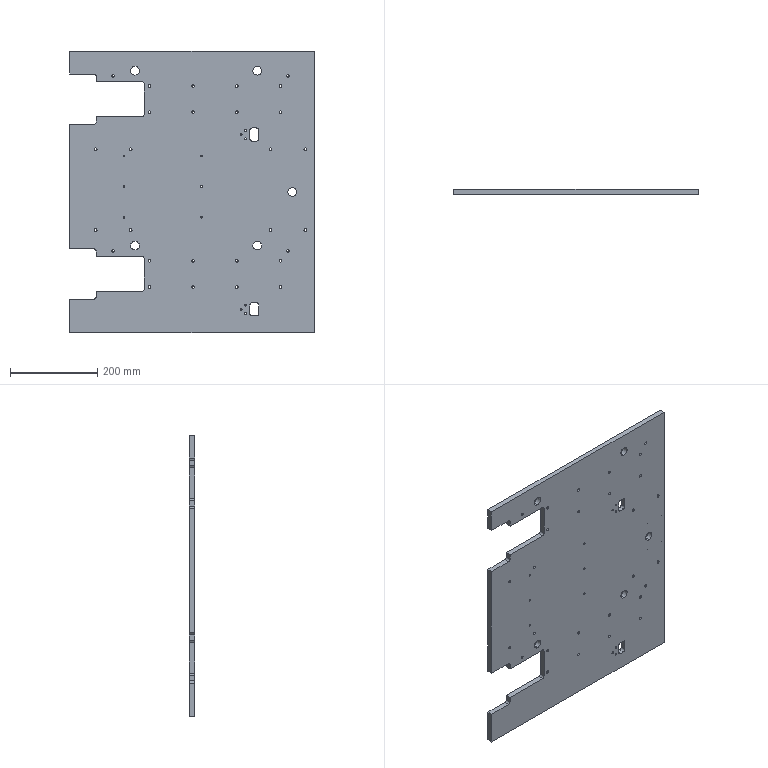Part | SolidWorks | features Cut 7, 3DProfileFeature 4, HoleWzd 4, Fillet 2, Extrusion 1, LPattern 1 | 1 solid | 176 faces | box 559 x 12 x 645 mm | volume 3901978 mm3 | cylinder 130 | plane 38 | cone 8 | commonest cylinder face diameters 6 x40 4.2 x24 6.6 x16 10 x16 11 x16 20 x10